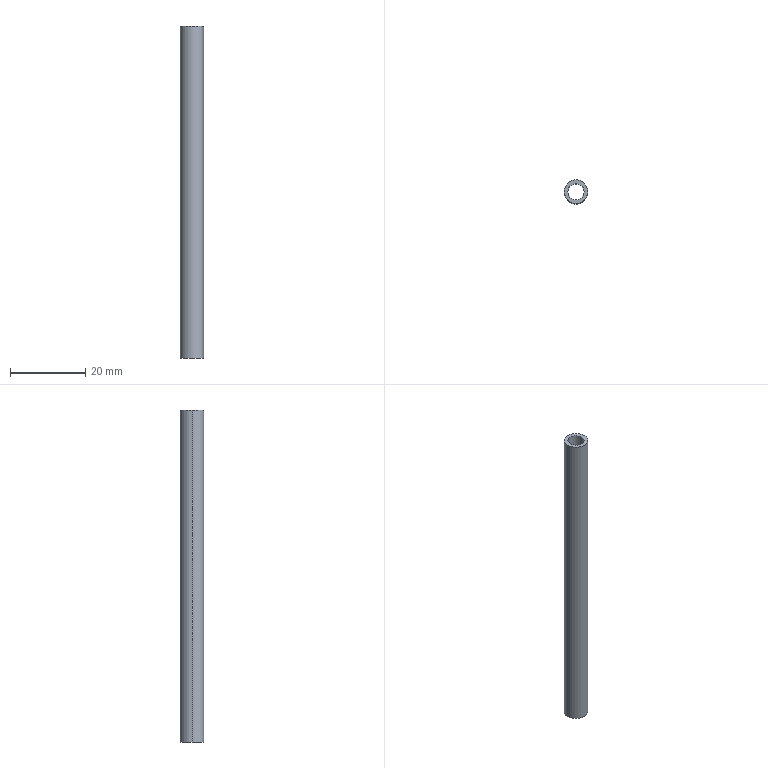Part | STEP file | Spring | 1 solid | 6 faces | box 6.3 x 6.3 x 88.5 mm | volume 1474 mm3 | cylinder 4 | plane 2 | commonest cylinder face diameters 4.3 x2 6.3 x2
STEP:
#1=CARTESIAN_POINT('',(0.,0.,0.));
#2=DIRECTION('',(0.,0.,1.));
#3=DIRECTION('',(1.,0.,0.));
#4=AXIS2_PLACEMENT_3D('',#1,#2,#3);
#5=CARTESIAN_POINT('',(-2.15,0.,44.25));
#6=VERTEX_POINT('',#5);
#7=CARTESIAN_POINT('',(-2.15,0.,-44.25));
#8=VERTEX_POINT('',#7);
#9=CARTESIAN_POINT('',(-2.15,0.,44.25));
#10=DIRECTION('',(0.,0.,-1.));
#11=VECTOR('',#10,1.);
#12=LINE('',#9,#11);
#13=CARTESIAN_POINT('',(0.,0.,44.25));
#14=DIRECTION('',(0.,0.,-1.));
#15=DIRECTION('',(-1.,0.,0.));
#16=AXIS2_PLACEMENT_3D('',#13,#14,#15);
#17=CYLINDRICAL_SURFACE('',#16,2.15);
#18=CARTESIAN_POINT('',(6.283,0.));
#19=DIRECTION('',(0.,1.));
#20=VECTOR('',#19,1.);
#21=LINE('',#18,#20);
#22=(GEOMETRIC_REPRESENTATION_CONTEXT(2)PARAMETRIC_REPRESENTATION_CONTEXT()REPRESENTATION_CONTEXT('',''));
#23=DEFINITIONAL_REPRESENTATION('',(#21),#22);
#24=PCURVE('',#17,#23);
#25=CARTESIAN_POINT('',(0.,0.,44.25));
#26=DIRECTION('',(0.,0.,-1.));
#27=DIRECTION('',(-1.,0.,0.));
#28=AXIS2_PLACEMENT_3D('',#25,#26,#27);
#29=CYLINDRICAL_SURFACE('',#28,2.15);
#30=CARTESIAN_POINT('',(0.,0.));
#31=DIRECTION('',(0.,1.));
#32=VECTOR('',#31,1.);
#33=LINE('',#30,#32);
#34=(GEOMETRIC_REPRESENTATION_CONTEXT(2)PARAMETRIC_REPRESENTATION_CONTEXT()REPRESENTATION_CONTEXT('',''));
#35=DEFINITIONAL_REPRESENTATION('',(#33),#34);
#36=PCURVE('',#29,#35);
#37=SURFACE_CURVE('',#12,(#24,#36),.PCURVE_S1.);
#38=EDGE_CURVE('',#6,#8,#37,.T.);
#39=ORIENTED_EDGE('',*,*,#38,.T.);
#40=CARTESIAN_POINT('',(2.15,0.,-44.25));
#41=VERTEX_POINT('',#40);
#42=CARTESIAN_POINT('',(0.,0.,-44.25));
#43=DIRECTION('',(0.,0.,1.));
#44=DIRECTION('',(1.,0.,0.));
#45=AXIS2_PLACEMENT_3D('',#42,#43,#44);
#46=CIRCLE('',#45,2.15);
#47=CARTESIAN_POINT('',(9.425,88.5));
#48=DIRECTION('',(-1.,0.));
#49=VECTOR('',#48,1.);
#50=LINE('',#47,#49);
#51=(GEOMETRIC_REPRESENTATION_CONTEXT(2)PARAMETRIC_REPRESENTATION_CONTEXT()REPRESENTATION_CONTEXT('',''));
#52=DEFINITIONAL_REPRESENTATION('',(#50),#51);
#53=PCURVE('',#17,#52);
#54=CARTESIAN_POINT('',(0.,0.,-44.25));
#55=DIRECTION('',(0.,0.,1.));
#56=DIRECTION('',(1.,0.,0.));
#57=AXIS2_PLACEMENT_3D('',#54,#55,#56);
#58=PLANE('',#57);
#59=CARTESIAN_POINT('',(0.,0.));
#60=DIRECTION('',(1.,0.));
#61=AXIS2_PLACEMENT_2D('',#59,#60);
#62=CIRCLE('',#61,2.15);
#63=(GEOMETRIC_REPRESENTATION_CONTEXT(2)PARAMETRIC_REPRESENTATION_CONTEXT()REPRESENTATION_CONTEXT('',''));
#64=DEFINITIONAL_REPRESENTATION('',(#62),#63);
#65=PCURVE('',#58,#64);
#66=SURFACE_CURVE('',#46,(#53,#65),.PCURVE_S1.);
#67=EDGE_CURVE('',#8,#41,#66,.T.);
#68=ORIENTED_EDGE('',*,*,#67,.T.);
#69=CARTESIAN_POINT('',(2.15,0.,44.25));
#70=VERTEX_POINT('',#69);
#71=CARTESIAN_POINT('',(2.15,0.,44.25));
#72=DIRECTION('',(0.,0.,-1.));
#73=VECTOR('',#72,1.);
#74=LINE('',#71,#73);
#75=CARTESIAN_POINT('',(3.142,0.));
#76=DIRECTION('',(0.,1.));
#77=VECTOR('',#76,1.);
#78=LINE('',#75,#77);
#79=(GEOMETRIC_REPRESENTATION_CONTEXT(2)PARAMETRIC_REPRESENTATION_CONTEXT()REPRESENTATION_CONTEXT('',''));
#80=DEFINITIONAL_REPRESENTATION('',(#78),#79);
#81=PCURVE('',#17,#80);
#82=CARTESIAN_POINT('',(3.142,0.));
#83=DIRECTION('',(0.,1.));
#84=VECTOR('',#83,1.);
#85=LINE('',#82,#84);
#86=(GEOMETRIC_REPRESENTATION_CONTEXT(2)PARAMETRIC_REPRESENTATION_CONTEXT()REPRESENTATION_CONTEXT('',''));
#87=DEFINITIONAL_REPRESENTATION('',(#85),#86);
#88=PCURVE('',#29,#87);
#89=SURFACE_CURVE('',#74,(#81,#88),.PCURVE_S1.);
#90=EDGE_CURVE('',#70,#41,#89,.T.);
#91=ORIENTED_EDGE('',*,*,#90,.F.);
#92=CARTESIAN_POINT('',(0.,0.,44.25));
#93=DIRECTION('',(0.,0.,1.));
#94=DIRECTION('',(1.,0.,0.));
#95=AXIS2_PLACEMENT_3D('',#92,#93,#94);
#96=CIRCLE('',#95,2.15);
#97=CARTESIAN_POINT('',(9.425,0.));
#98=DIRECTION('',(-1.,0.));
#99=VECTOR('',#98,1.);
#100=LINE('',#97,#99);
#101=(GEOMETRIC_REPRESENTATION_CONTEXT(2)PARAMETRIC_REPRESENTATION_CONTEXT()REPRESENTATION_CONTEXT('',''));
#102=DEFINITIONAL_REPRESENTATION('',(#100),#101);
#103=PCURVE('',#17,#102);
#104=CARTESIAN_POINT('',(0.,0.,44.25));
#105=DIRECTION('',(0.,0.,1.));
#106=DIRECTION('',(1.,0.,0.));
#107=AXIS2_PLACEMENT_3D('',#104,#105,#106);
#108=PLANE('',#107);
#109=CARTESIAN_POINT('',(0.,0.));
#110=DIRECTION('',(1.,0.));
#111=AXIS2_PLACEMENT_2D('',#109,#110);
#112=CIRCLE('',#111,2.15);
#113=(GEOMETRIC_REPRESENTATION_CONTEXT(2)PARAMETRIC_REPRESENTATION_CONTEXT()REPRESENTATION_CONTEXT('',''));
#114=DEFINITIONAL_REPRESENTATION('',(#112),#113);
#115=PCURVE('',#108,#114);
#116=SURFACE_CURVE('',#96,(#103,#115),.PCURVE_S1.);
#117=EDGE_CURVE('',#6,#70,#116,.T.);
#118=ORIENTED_EDGE('',*,*,#117,.F.);
#119=EDGE_LOOP('',(#39,#68,#91,#118));
#120=FACE_BOUND('',#119,.F.);
#121=ADVANCED_FACE('',(#120),#17,.F.);
#122=CARTESIAN_POINT('',(3.15,0.,44.25));
#123=VERTEX_POINT('',#122);
#124=CARTESIAN_POINT('',(-3.15,0.,44.25));
#125=VERTEX_POINT('',#124);
#126=CARTESIAN_POINT('',(0.,0.,44.25));
#127=DIRECTION('',(0.,0.,1.));
#128=DIRECTION('',(1.,0.,0.));
#129=AXIS2_PLACEMENT_3D('',#126,#127,#128);
#130=CIRCLE('',#129,3.15);
#131=CARTESIAN_POINT('',(0.,0.,44.25));
#132=DIRECTION('',(0.,0.,-1.));
#133=DIRECTION('',(-1.,0.,0.));
#134=AXIS2_PLACEMENT_3D('',#131,#132,#133);
#135=CYLINDRICAL_SURFACE('',#134,3.15);
#136=CARTESIAN_POINT('',(3.142,0.));
#137=DIRECTION('',(-1.,0.));
#138=VECTOR('',#137,1.);
#139=LINE('',#136,#138);
#140=(GEOMETRIC_REPRESENTATION_CONTEXT(2)PARAMETRIC_REPRESENTATION_CONTEXT()REPRESENTATION_CONTEXT('',''));
#141=DEFINITIONAL_REPRESENTATION('',(#139),#140);
#142=PCURVE('',#135,#141);
#143=CARTESIAN_POINT('',(0.,0.));
#144=DIRECTION('',(1.,0.));
#145=AXIS2_PLACEMENT_2D('',#143,#144);
#146=CIRCLE('',#145,3.15);
#147=(GEOMETRIC_REPRESENTATION_CONTEXT(2)PARAMETRIC_REPRESENTATION_CONTEXT()REPRESENTATION_CONTEXT('',''));
#148=DEFINITIONAL_REPRESENTATION('',(#146),#147);
#149=PCURVE('',#108,#148);
#150=SURFACE_CURVE('',#130,(#142,#149),.PCURVE_S1.);
#151=EDGE_CURVE('',#123,#125,#150,.T.);
#152=ORIENTED_EDGE('',*,*,#151,.F.);
#153=CARTESIAN_POINT('',(3.15,0.,-44.25));
#154=VERTEX_POINT('',#153);
#155=CARTESIAN_POINT('',(3.15,0.,44.25));
#156=DIRECTION('',(0.,0.,-1.));
#157=VECTOR('',#156,1.);
#158=LINE('',#155,#157);
#159=CARTESIAN_POINT('',(3.142,0.));
#160=DIRECTION('',(0.,1.));
#161=VECTOR('',#160,1.);
#162=LINE('',#159,#161);
#163=(GEOMETRIC_REPRESENTATION_CONTEXT(2)PARAMETRIC_REPRESENTATION_CONTEXT()REPRESENTATION_CONTEXT('',''));
#164=DEFINITIONAL_REPRESENTATION('',(#162),#163);
#165=PCURVE('',#135,#164);
#166=CARTESIAN_POINT('',(0.,0.,44.25));
#167=DIRECTION('',(0.,0.,-1.));
#168=DIRECTION('',(-1.,0.,0.));
#169=AXIS2_PLACEMENT_3D('',#166,#167,#168);
#170=CYLINDRICAL_SURFACE('',#169,3.15);
#171=CARTESIAN_POINT('',(3.142,0.));
#172=DIRECTION('',(0.,1.));
#173=VECTOR('',#172,1.);
#174=LINE('',#171,#173);
#175=(GEOMETRIC_REPRESENTATION_CONTEXT(2)PARAMETRIC_REPRESENTATION_CONTEXT()REPRESENTATION_CONTEXT('',''));
#176=DEFINITIONAL_REPRESENTATION('',(#174),#175);
#177=PCURVE('',#170,#176);
#178=SURFACE_CURVE('',#158,(#165,#177),.PCURVE_S1.);
#179=EDGE_CURVE('',#123,#154,#178,.T.);
#180=ORIENTED_EDGE('',*,*,#179,.T.);
#181=CARTESIAN_POINT('',(-3.15,0.,-44.25));
#182=VERTEX_POINT('',#181);
#183=CARTESIAN_POINT('',(0.,0.,-44.25));
#184=DIRECTION('',(0.,0.,1.));
#185=DIRECTION('',(1.,0.,0.));
#186=AXIS2_PLACEMENT_3D('',#183,#184,#185);
#187=CIRCLE('',#186,3.15);
#188=CARTESIAN_POINT('',(3.142,88.5));
#189=DIRECTION('',(-1.,0.));
#190=VECTOR('',#189,1.);
#191=LINE('',#188,#190);
#192=(GEOMETRIC_REPRESENTATION_CONTEXT(2)PARAMETRIC_REPRESENTATION_CONTEXT()REPRESENTATION_CONTEXT('',''));
#193=DEFINITIONAL_REPRESENTATION('',(#191),#192);
#194=PCURVE('',#135,#193);
#195=CARTESIAN_POINT('',(0.,0.));
#196=DIRECTION('',(1.,0.));
#197=AXIS2_PLACEMENT_2D('',#195,#196);
#198=CIRCLE('',#197,3.15);
#199=(GEOMETRIC_REPRESENTATION_CONTEXT(2)PARAMETRIC_REPRESENTATION_CONTEXT()REPRESENTATION_CONTEXT('',''));
#200=DEFINITIONAL_REPRESENTATION('',(#198),#199);
#201=PCURVE('',#58,#200);
#202=SURFACE_CURVE('',#187,(#194,#201),.PCURVE_S1.);
#203=EDGE_CURVE('',#154,#182,#202,.T.);
#204=ORIENTED_EDGE('',*,*,#203,.T.);
#205=CARTESIAN_POINT('',(-3.15,0.,44.25));
#206=DIRECTION('',(0.,0.,-1.));
#207=VECTOR('',#206,1.);
#208=LINE('',#205,#207);
#209=CARTESIAN_POINT('',(0.,0.));
#210=DIRECTION('',(0.,1.));
#211=VECTOR('',#210,1.);
#212=LINE('',#209,#211);
#213=(GEOMETRIC_REPRESENTATION_CONTEXT(2)PARAMETRIC_REPRESENTATION_CONTEXT()REPRESENTATION_CONTEXT('',''));
#214=DEFINITIONAL_REPRESENTATION('',(#212),#213);
#215=PCURVE('',#135,#214);
#216=CARTESIAN_POINT('',(6.283,0.));
#217=DIRECTION('',(0.,1.));
#218=VECTOR('',#217,1.);
#219=LINE('',#216,#218);
#220=(GEOMETRIC_REPRESENTATION_CONTEXT(2)PARAMETRIC_REPRESENTATION_CONTEXT()REPRESENTATION_CONTEXT('',''));
#221=DEFINITIONAL_REPRESENTATION('',(#219),#220);
#222=PCURVE('',#170,#221);
#223=SURFACE_CURVE('',#208,(#215,#222),.PCURVE_S1.);
#224=EDGE_CURVE('',#125,#182,#223,.T.);
#225=ORIENTED_EDGE('',*,*,#224,.F.);
#226=EDGE_LOOP('',(#152,#180,#204,#225));
#227=FACE_BOUND('',#226,.T.);
#228=ADVANCED_FACE('',(#227),#135,.T.);
#229=CARTESIAN_POINT('',(0.,0.,44.25));
#230=DIRECTION('',(0.,0.,1.));
#231=DIRECTION('',(1.,0.,0.));
#232=AXIS2_PLACEMENT_3D('',#229,#230,#231);
#233=CIRCLE('',#232,3.15);
#234=CARTESIAN_POINT('',(0.,0.));
#235=DIRECTION('',(1.,0.));
#236=AXIS2_PLACEMENT_2D('',#234,#235);
#237=CIRCLE('',#236,3.15);
#238=(GEOMETRIC_REPRESENTATION_CONTEXT(2)PARAMETRIC_REPRESENTATION_CONTEXT()REPRESENTATION_CONTEXT('',''));
#239=DEFINITIONAL_REPRESENTATION('',(#237),#238);
#240=PCURVE('',#108,#239);
#241=CARTESIAN_POINT('',(9.425,0.));
#242=DIRECTION('',(-1.,0.));
#243=VECTOR('',#242,1.);
#244=LINE('',#241,#243);
#245=(GEOMETRIC_REPRESENTATION_CONTEXT(2)PARAMETRIC_REPRESENTATION_CONTEXT()REPRESENTATION_CONTEXT('',''));
#246=DEFINITIONAL_REPRESENTATION('',(#244),#245);
#247=PCURVE('',#170,#246);
#248=SURFACE_CURVE('',#233,(#240,#247),.PCURVE_S1.);
#249=EDGE_CURVE('',#125,#123,#248,.T.);
#250=ORIENTED_EDGE('',*,*,#249,.T.);
#251=ORIENTED_EDGE('',*,*,#151,.T.);
#252=EDGE_LOOP('',(#250,#251));
#253=FACE_BOUND('',#252,.T.);
#254=ORIENTED_EDGE('',*,*,#117,.F.);
#255=CARTESIAN_POINT('',(0.,0.,44.25));
#256=DIRECTION('',(0.,0.,1.));
#257=DIRECTION('',(1.,0.,0.));
#258=AXIS2_PLACEMENT_3D('',#255,#256,#257);
#259=CIRCLE('',#258,2.15);
#260=CARTESIAN_POINT('',(0.,0.));
#261=DIRECTION('',(1.,0.));
#262=AXIS2_PLACEMENT_2D('',#260,#261);
#263=CIRCLE('',#262,2.15);
#264=(GEOMETRIC_REPRESENTATION_CONTEXT(2)PARAMETRIC_REPRESENTATION_CONTEXT()REPRESENTATION_CONTEXT('',''));
#265=DEFINITIONAL_REPRESENTATION('',(#263),#264);
#266=PCURVE('',#108,#265);
#267=CARTESIAN_POINT('',(3.142,0.));
#268=DIRECTION('',(-1.,0.));
#269=VECTOR('',#268,1.);
#270=LINE('',#267,#269);
#271=(GEOMETRIC_REPRESENTATION_CONTEXT(2)PARAMETRIC_REPRESENTATION_CONTEXT()REPRESENTATION_CONTEXT('',''));
#272=DEFINITIONAL_REPRESENTATION('',(#270),#271);
#273=PCURVE('',#29,#272);
#274=SURFACE_CURVE('',#259,(#266,#273),.PCURVE_S1.);
#275=EDGE_CURVE('',#70,#6,#274,.T.);
#276=ORIENTED_EDGE('',*,*,#275,.F.);
#277=EDGE_LOOP('',(#254,#276));
#278=FACE_BOUND('',#277,.T.);
#279=ADVANCED_FACE('',(#253,#278),#108,.T.);
#280=CARTESIAN_POINT('',(0.,0.,-44.25));
#281=DIRECTION('',(0.,0.,1.));
#282=DIRECTION('',(1.,0.,0.));
#283=AXIS2_PLACEMENT_3D('',#280,#281,#282);
#284=CIRCLE('',#283,3.15);
#285=CARTESIAN_POINT('',(0.,0.));
#286=DIRECTION('',(1.,0.));
#287=AXIS2_PLACEMENT_2D('',#285,#286);
#288=CIRCLE('',#287,3.15);
#289=(GEOMETRIC_REPRESENTATION_CONTEXT(2)PARAMETRIC_REPRESENTATION_CONTEXT()REPRESENTATION_CONTEXT('',''));
#290=DEFINITIONAL_REPRESENTATION('',(#288),#289);
#291=PCURVE('',#58,#290);
#292=CARTESIAN_POINT('',(9.425,88.5));
#293=DIRECTION('',(-1.,0.));
#294=VECTOR('',#293,1.);
#295=LINE('',#292,#294);
#296=(GEOMETRIC_REPRESENTATION_CONTEXT(2)PARAMETRIC_REPRESENTATION_CONTEXT()REPRESENTATION_CONTEXT('',''));
#297=DEFINITIONAL_REPRESENTATION('',(#295),#296);
#298=PCURVE('',#170,#297);
#299=SURFACE_CURVE('',#284,(#291,#298),.PCURVE_S1.);
#300=EDGE_CURVE('',#182,#154,#299,.T.);
#301=ORIENTED_EDGE('',*,*,#300,.F.);
#302=ORIENTED_EDGE('',*,*,#203,.F.);
#303=EDGE_LOOP('',(#301,#302));
#304=FACE_BOUND('',#303,.T.);
#305=ORIENTED_EDGE('',*,*,#67,.T.);
#306=CARTESIAN_POINT('',(0.,0.,-44.25));
#307=DIRECTION('',(0.,0.,1.));
#308=DIRECTION('',(1.,0.,0.));
#309=AXIS2_PLACEMENT_3D('',#306,#307,#308);
#310=CIRCLE('',#309,2.15);
#311=CARTESIAN_POINT('',(0.,0.));
#312=DIRECTION('',(1.,0.));
#313=AXIS2_PLACEMENT_2D('',#311,#312);
#314=CIRCLE('',#313,2.15);
#315=(GEOMETRIC_REPRESENTATION_CONTEXT(2)PARAMETRIC_REPRESENTATION_CONTEXT()REPRESENTATION_CONTEXT('',''));
#316=DEFINITIONAL_REPRESENTATION('',(#314),#315);
#317=PCURVE('',#58,#316);
#318=CARTESIAN_POINT('',(3.142,88.5));
#319=DIRECTION('',(-1.,0.));
#320=VECTOR('',#319,1.);
#321=LINE('',#318,#320);
#322=(GEOMETRIC_REPRESENTATION_CONTEXT(2)PARAMETRIC_REPRESENTATION_CONTEXT()REPRESENTATION_CONTEXT('',''));
#323=DEFINITIONAL_REPRESENTATION('',(#321),#322);
#324=PCURVE('',#29,#323);
#325=SURFACE_CURVE('',#310,(#317,#324),.PCURVE_S1.);
#326=EDGE_CURVE('',#41,#8,#325,.T.);
#327=ORIENTED_EDGE('',*,*,#326,.T.);
#328=EDGE_LOOP('',(#305,#327));
#329=FACE_BOUND('',#328,.T.);
#330=ADVANCED_FACE('',(#304,#329),#58,.F.);
#331=ORIENTED_EDGE('',*,*,#179,.F.);
#332=ORIENTED_EDGE('',*,*,#249,.F.);
#333=ORIENTED_EDGE('',*,*,#224,.T.);
#334=ORIENTED_EDGE('',*,*,#300,.T.);
#335=EDGE_LOOP('',(#331,#332,#333,#334));
#336=FACE_BOUND('',#335,.T.);
#337=ADVANCED_FACE('',(#336),#170,.T.);
#338=ORIENTED_EDGE('',*,*,#326,.T.);
#339=ORIENTED_EDGE('',*,*,#38,.F.);
#340=ORIENTED_EDGE('',*,*,#275,.F.);
#341=ORIENTED_EDGE('',*,*,#90,.T.);
#342=EDGE_LOOP('',(#338,#339,#340,#341));
#343=FACE_BOUND('',#342,.F.);
#344=ADVANCED_FACE('',(#343),#29,.F.);
#345=CLOSED_SHELL('',(#121,#228,#279,#330,#337,#344));
#346=MANIFOLD_SOLID_BREP('',#345);
#347=(LENGTH_UNIT()NAMED_UNIT(*)SI_UNIT(.MILLI.,.METRE.));
#348=UNCERTAINTY_MEASURE_WITH_UNIT(LENGTH_MEASURE(0.0000001),#347,'','');
#349=(NAMED_UNIT(*)PLANE_ANGLE_UNIT()SI_UNIT($,.RADIAN.));
#350=(NAMED_UNIT(*)SI_UNIT($,.STERADIAN.)SOLID_ANGLE_UNIT());
#351=(GEOMETRIC_REPRESENTATION_CONTEXT(3)GLOBAL_UNCERTAINTY_ASSIGNED_CONTEXT((#348))GLOBAL_UNIT_ASSIGNED_CONTEXT((#347,#349,#350))REPRESENTATION_CONTEXT('',''));
#352=ADVANCED_BREP_SHAPE_REPRESENTATION('',(#4,#346),#351);